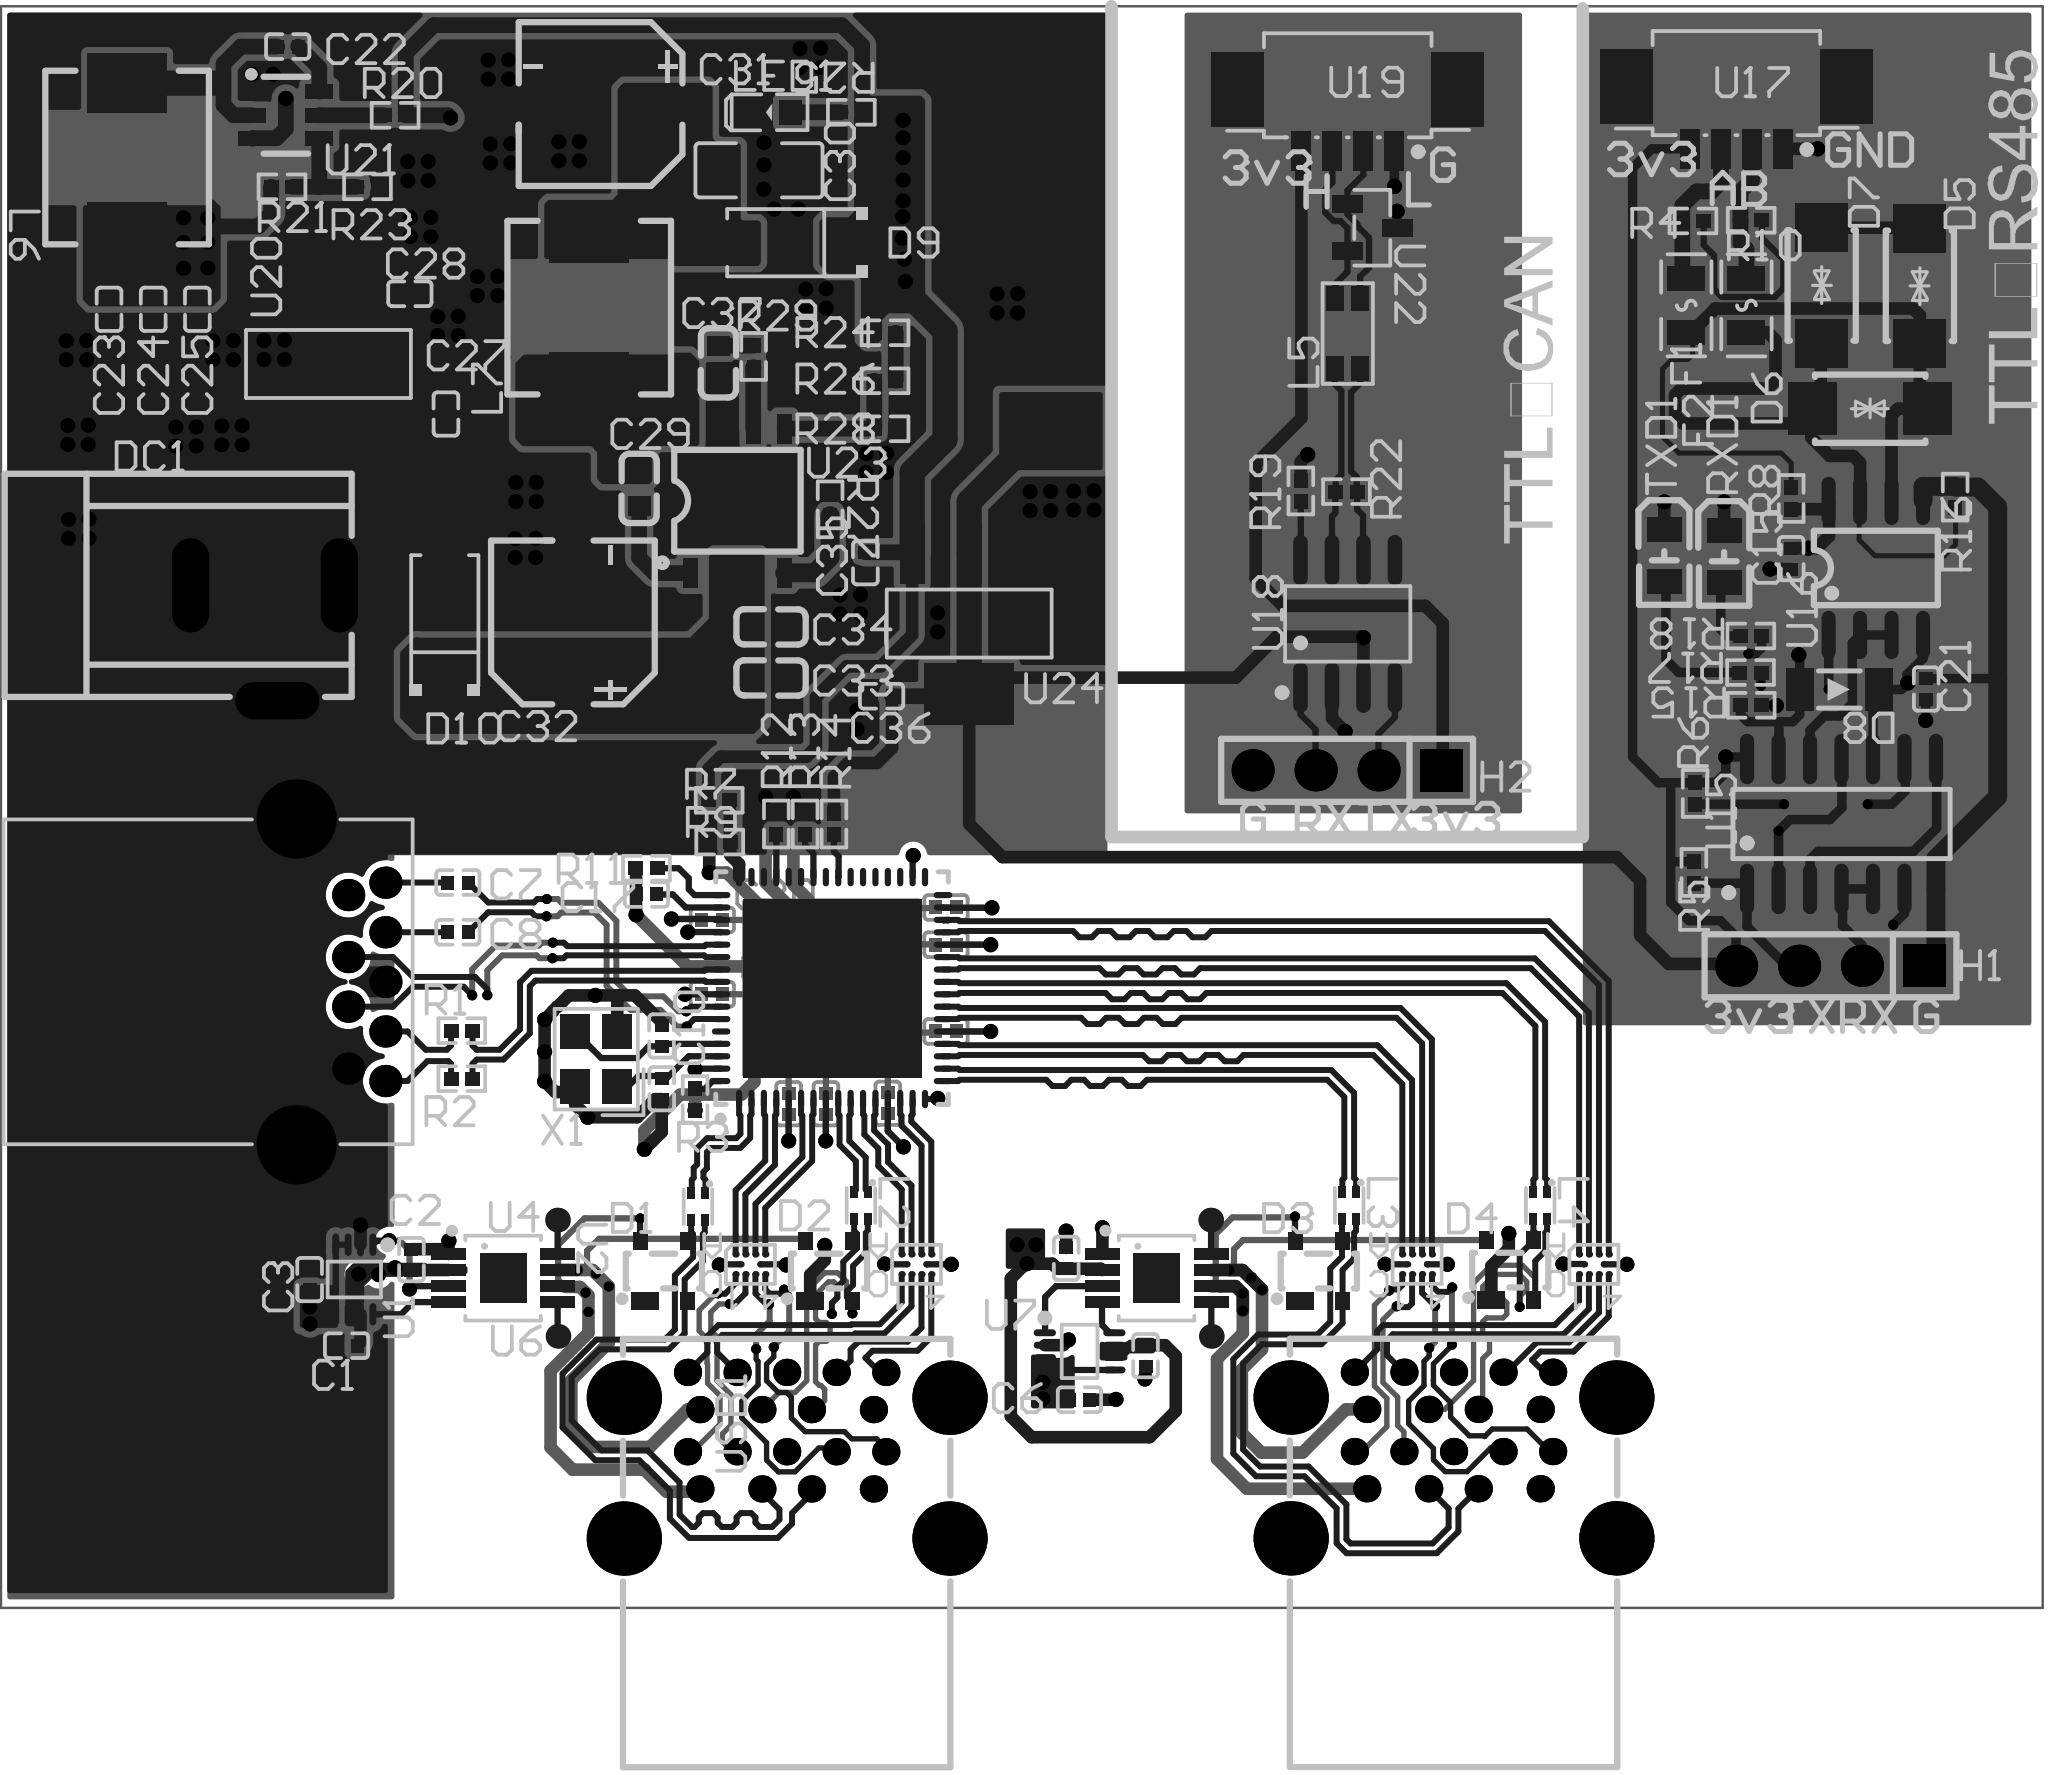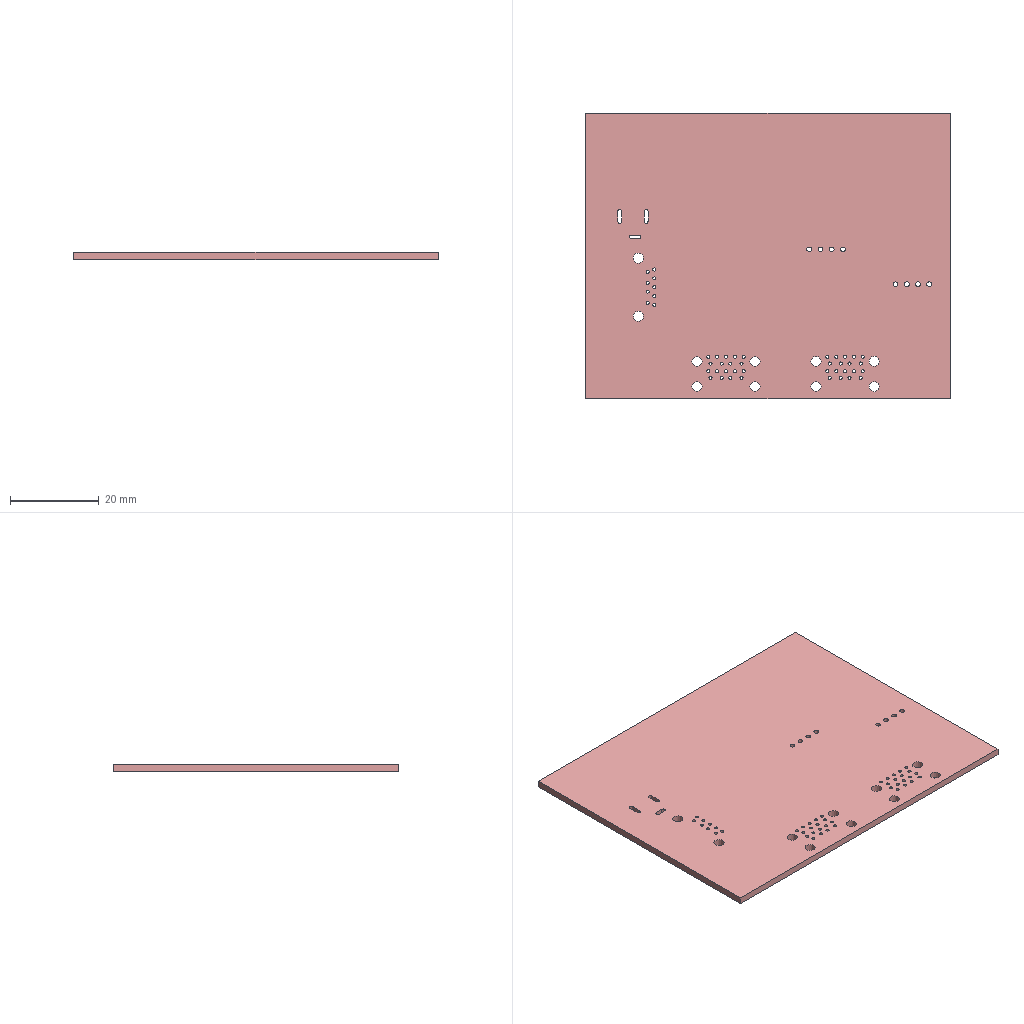Circuit board layout | Altium Designer | box 82.4 x 64.6 x 1.6 mm
Layer stack:
# Altium Designer layer stack of  (unit mm; dielectric type: 0 none, 1 core, 2 prepreg, 3 surface material)
index,name,kind,layer,copper_thickness_mm,dielectric_type,dielectric_thickness_mm,dielectric_material,dielectric_constant
0,Top Paste Mask Layer,other,,,,,,
1,Top Silkscreen Layer,other,,,,,,
2,Top Solder Mask Layer,dielectric,,,3,0,,0
3,Top Layer,copper,Top Layer,0.035,,,,
4,Dielectric1,dielectric,,,3,0.2104,7628 RC49% 8.6mil,0
5,GND,copper,GND,0.0152,,,,
6,Dielectric2,dielectric,,,3,1.065,1.1mm H/HOZ Copper,0
7,Signal-1,copper,Signal-1,0.0152,,,,
8,Dielectric3,dielectric,,,3,0.2104,7628 RC49% 8.6mil,0
9,Bottom Layer,copper,Bottom Layer,0.035,,,,
10,Bottom Solder Mask Layer,dielectric,,,3,0,,0
11,Bottom Silkscreen Layer,other,,,,,,
12,Bottom Paste Mask Layer,other,,,,,,
# drill layer pairs: low layer,high layer
drill_pair,Top Layer,Bottom Layer
Part placement:
Designator,Comment,Layer,Footprint,Center-X(mm),Center-Y(mm),Rotation
USB2,HC-USB3.0-L175-2X1-P,TopLayer,USB-A-TH_H181-AF2R06-12ALCR,134.993,88.908,0
U14,TUSB8041IRGCR,TopLayer,QFN-64_L9.0-W9.0-P0.50-BL-EP7.2,109.921,107.749,0
D4,CD143A-SR05,TopLayer,SOT-143_L2.9-W1.3-P1.92-LS2.3-BL,137.269,96.375,0
USB1,HC-USB3.0-L175-2X1-P,TopLayer,USB-A-TH_H181-AF2R06-12ALCR,108.09,88.9,0
L1,DLM11SN900HY2L,TopLayer,FILTER-SMD_4P-L1.3-W1.0-TL_DLP11SN201HL2L,104.511,98.936,270
U11,,TopLayer,PCMF2USB3S,133.524,96.609,90
C5,100nF,TopLayer,C0402,119.367,96.85,90
L3,DLM11SN900HY2L,TopLayer,FILTER-SMD_4P-L1.3-W1.0-TL_DLP11SN201HL2L,130.785,98.986,270
C31,220uF,TopLayer,CAP-SMD_BD6.3-L6.5-W6.5-LS7.2-FD,100.581,143.401,180
C32,100uF,TopLayer,CAP-SMD_BD6.3-L6.5-W6.5-LS7.0-FD,99.466,122.497,90
C30,47uF,TopLayer,C1206,106.972,140.729,180
C29,100nF,TopLayer,C0603,102.136,127.893,270
C34,100nF,TopLayer,C0603,107.452,122.319,180
C37,4.7nF,TopLayer,C0603,105.334,132.956,270
C33,4.7uF,TopLayer,C0603,107.452,120.259,180
D9,SS54,TopLayer,SMA_L4.4-W2.8-LS5.4-R-RD,108.336,137.81,180
D10,SS54,TopLayer,SMA_L4.4-W2.8-LS5.4-R-RD,94.297,122.563,90
D1,CD143A-SR05,TopLayer,SOT-143_L2.9-W1.3-P1.92-LS2.3-BL,103.124,96.337,0
D2,CD143A-SR05,TopLayer,SOT-143_L2.9-W1.3-P1.92-LS2.3-BL,109.789,96.337,0
D3,CD143A-SR05,TopLayer,SOT-143_L2.9-W1.3-P1.92-LS2.3-BL,129.548,96.337,0
D8,LL4148,TopLayer,LL-34_L3.5-W1.5-RD,150.557,119.791,180
D5,SMAJ6.5CA,TopLayer,SMA-L4.3-W2.6-LS5.3-BI,153.808,136.072,90
D7,SMAJ6.5CA,TopLayer,SMA-L4.3-W2.6-LS5.3-BI,149.846,136.085,270
D6,SMAJ6.5CA,TopLayer,SMA-L4.3-W2.6-LS5.3-BI,151.803,131.115,0
DC1,DC-005-A200,TopLayer,DC-IN-TH_DC-005-A200,87.041,121.666,0
H2,PZ254V-11-04P,TopLayer,HDR-TH_4P-P2.54-V-M,130.699,116.532,180
H1,PZ254V-11-04P,TopLayer,HDR-TH_4P-P2.54-V-M,150.203,108.648,180
L7,4.7uH,TopLayer,IND-SMD_L7.0-W6.6,100.124,135.192,90
L6,3.3uH,TopLayer,IND-SMD_L7.0-W6.6,81.481,141.244,90
L2,DLM11SN900HY2L,TopLayer,FILTER-SMD_4P-L1.3-W1.0-TL_DLP11SN201HL2L,111.087,98.986,270
L4,DLM11SN900HY2L,TopLayer,FILTER-SMD_4P-L1.3-W1.0-TL_DLP11SN201HL2L,138.491,98.986,270
L5,744232102,TopLayer,IND-SMD_4P-L3.2-W1.6,130.725,134.147,90
LED1,15-21VGC/TR8,TopLayer,LED0603_GREEN,107.391,143.071,180
RXD1,GL0805UR01,TopLayer,LED0805-R-RD_RED,145.909,125.163,270
TXD1,GL0805UR01,TopLayer,LED0805-R-RD_RED,143.496,125.201,270
U23,SCT2450STER,TopLayer,ESOP-8_L4.9-W3.9-P1.27-LS6.0-BL-EP,106.103,127.404,0
U21,TPS563201DDCR,TopLayer,SOT-23-6_L2.9-W1.6-P0.95-LS2.8-BR,87.884,142.951,180
U2,TPS2060CDGNR,TopLayer,HVSSOP-8_L3.0-W3.0-P0.65-LS4.9-BL-EP-1,96.65,96.053,270
U1,TXS0102DCUT,TopLayer,VSSOP-8_L2.3-W2.0-P0.50-LS3.1-BR,90.647,95.997,90
U8,TPS2060CDGNR,TopLayer,HVSSOP-8_L3.0-W3.0-P0.65-LS4.9-BL-EP-1,123.012,96.053,270
U7,TXS0102DCUT,TopLayer,VSSOP-8_L2.3-W2.0-P0.50-LS3.1-BR,119.908,93.098,180
U3,,TopLayer,PCMF2USB3S,113.329,96.609,90
U9,,TopLayer,PCMF2USB3S,140.658,96.609,90
U5,,TopLayer,PCMF2USB3S,106.629,96.609,90
U16,SP3485EN-L/TR,TopLayer,SOIC-8_L5.0-W4.0-P1.27-LS6.0-BL,152.03,124.693,0
U15,74HC04D,653,TopLayer,SOIC-14_L8.7-W3.9-P1.27-LS6.0-BL,150.646,114.368,0
U17,ZX-MX1.25-4PWT,TopLayer,CONN-SMD_4P-P1.25-MX1.25-4P-WT,146.404,142.846,180
U19,ZX-MX1.25-4PWT,TopLayer,CONN-SMD_4P-P1.25-MX1.25-4P-WT,130.725,142.757,180
U18,SN65HVD230DR,TopLayer,SOIC-8_L4.9-W3.9-P1.27-LS6.0-BL,130.725,122.437,0
U22,SM24CANA-02HTG,TopLayer,SOT-23-3_L2.9-W1.3-P1.90-LS2.4-BR,131.715,138.414,180
U13,HC-USB3.0-L168-WP,TopLayer,USB-TH_USB3.0-A,90.1,108.001,270
U20,AMS1117-1.8,TopLayer,SOT-223-4_L6.5-W3.5-P2.30-LS7.0-BR,89.604,132.918,270
U24,AMS1117-3.3,TopLayer,SOT-223-4_L6.5-W3.5-P2.30-LS7.0-BR,115.453,122.451,90
X1,24MHz,TopLayer,CRYSTAL-SMD_4P-L3.2-W2.5-BL,100.406,104.882,90
C22,100nF,TopLayer,C0402,87.96,145.72,0
C23,22uF,TopLayer,C0402,80.752,135.125,90
C24,22uF,TopLayer,C0402,82.534,135.125,90
C25,100nF,TopLayer,C0402,84.315,135.125,90
C10,12pF,TopLayer,C0402,103.04,105.819,270
C9,12pF,TopLayer,C0402,103.048,103.69,90
C17,100nF,TopLayer,C0402,102.433,111.524,180
C20,100nF,BottomLayer,C0402,105.09,110.498,180
C19,100nF,BottomLayer,C0402,109.672,103.086,270
C18,100nF,BottomLayer,C0402,114.517,109.499,0
C16,100nF,BottomLayer,C0402,114.517,111.001,0
C14,100nF,BottomLayer,C0402,114.517,105.999,0
C13,100nF,BottomLayer,C0402,112.169,103.104,270
C12,100nF,BottomLayer,C0402,105.09,107.5,180
C11,100nF,BottomLayer,C0402,108.168,103.086,270
C2,100nF,TopLayer,C0402,92.951,96.799,90
C1,100nF,TopLayer,C0402,90.335,93.327,0
C3,100nF,TopLayer,C0402,88.844,95.994,90
C4,100nF,TopLayer,C0402,122.568,92.926,90
C6,100nF,TopLayer,C0402,119.901,91.148,0
C15,Cap,TopLayer,C0402,148.615,125.07,270
C21,Cap,TopLayer,C0402,154.064,119.812,270
C8,100nF,TopLayer,C0402,94.825,110.002,0
C7,100nF,TopLayer,C0402,94.825,112.006,0
C28,22uF,TopLayer,C0402,92.888,135.75,180
C27,10uF,TopLayer,C0402,94.343,130.9,270
C36,22uF,TopLayer,C0402,111.92,119.52,0
C35,10uF,TopLayer,C0402,111.265,124.904,90
R26,1.5kΩ,TopLayer,R0402,112.057,132.241,180
R25,4.7kΩ,TopLayer,R0402,110.698,143.071,180
R28,10kΩ,TopLayer,R0402,112.057,130.304,0
R24,51kΩ,TopLayer,R0402,112.057,134.178,0
R29,20kΩ,TopLayer,R0402,106.756,133.223,90
R27,200kΩ,TopLayer,R0402,109.842,127.238,270
R20,10kΩ,TopLayer,R0402,92.293,142.949,0
R21,4.3kΩ,TopLayer,R0402,87.729,140.063,180
R23,10kΩ,TopLayer,R0402,91.178,140.063,0
R3,9.53K,TopLayer,R0402,104.394,103.251,270
R11,4.7K,TopLayer,R0402,102.433,112.583,180
R7,90.9K,TopLayer,R0402,105.367,115.323,180
R9,10K,TopLayer,R0402,105.389,113.637,180
R12,4.7K,TopLayer,R0402,107.673,114.366,90
R13,4.7K,TopLayer,R0402,108.834,114.366,90
R14,4.7K,TopLayer,R0402,109.997,114.366,90
R8,Res1,TopLayer,R0402,148.615,127.495,270
R16,Res1,TopLayer,R0402,155.231,127.549,270
R15,Res1,TopLayer,R0402,147.002,119.156,180
R17,Res1,TopLayer,R0402,146.976,120.476,180
R18,Res1,TopLayer,R0402,146.988,121.95,0
R5,Res1,TopLayer,R0402,144.69,112.412,90
R6,Res1,TopLayer,R0402,144.741,115.6,90
R10,Res1,TopLayer,R0402,147.001,138.714,0
R4,Res1,TopLayer,R0402,144.652,138.688,0
R19,10K,TopLayer,R0402,128.832,127.797,90
R22,120R 1%,TopLayer,R0402,130.674,127.771,180
R1,0R,TopLayer,R0402,94.982,106.032,0
R2,0R,TopLayer,R0402,94.982,104.096,0
U12,,TopLayer,tp点,125.222,93.703,180
U6,,TopLayer,tp点,98.864,93.703,0
U10,,TopLayer,tp点,125.197,98.394,180
U4,,TopLayer,tp点,98.844,98.394,0
F1,SMD0805-010-33,TopLayer,F0805,144.385,135.285,90
F2,SMD0805-010-33,TopLayer,F0805,146.811,135.285,90
Pad and via stacks:
# Altium Designer via and pad stacks of  (unit mm). Each distinct definition once, with the count of objects using it.
# via: kind,start_layer,end_layer,hole_mm,diameter_mm,mode(0 simple;1 top-mid-bottom;2 full stack),diameter_per_layer,count,example_net
# pad: kind,layer,hole_mm,hole_type(0 round;1 square;2 slot),plating,top_size,top_shape(1 round;2 rect;3 octagon;9 rounded rect),mid_size,bottom_size,mode,footprint,size_per_layer,count,example
pad,Multi-Layer,2.3,0,plated,3x3,1,3x3,3x3,0,USB-A-TH_H181-AF2R06-12ALCR,,8,USB2.20
pad,Multi-Layer,0.7,0,plated,1.1x1.1,1,1.1x1.1,1.1x1.1,0,USB-A-TH_H181-AF2R06-12ALCR,,36,USB2.18
pad,Multi-Layer,0.9,2,plated,1.5x3.8,1,1.5x3.8,1.5x3.8,0,DC-IN-TH_DC-005-A200,,2,DC1.1
pad,Multi-Layer,0.9,2,plated,1.5x3.4,1,1.5x3.4,1.5x3.4,0,DC-IN-TH_DC-005-A200,,1,DC1.3
pad,Multi-Layer,1.1,0,plated,1.7x1.7,2,1.7x1.7,1.7x1.7,0,HDR-TH_4P-P2.54-V-M,,2,H2.1
pad,Multi-Layer,1.1,0,plated,1.7x1.7,1,1.7x1.7,1.7x1.7,0,HDR-TH_4P-P2.54-V-M,,6,H2.2
pad,Multi-Layer,2.3,0,plated,3.2x3.2,1,3.2x3.2,3.2x3.2,0,USB-TH_USB3.0-A,,2,U13.10
pad,Multi-Layer,0.7,0,plated,1.3x1.3,1,1.3x1.3,1.3x1.3,0,USB-TH_USB3.0-A,,9,U13.9
pad,Top Layer,0,0,plated,0.25x0.75,1,0.25x0.75,0.25x0.75,0,QFN-64_L9.0-W9.0-P0.50-BL-EP7.2,,32,U14.1
pad,Top Layer,0,0,plated,7.2x7.2,2,7.2x7.2,7.2x7.2,0,QFN-64_L9.0-W9.0-P0.50-BL-EP7.2,,1,U14.65
pad,Top Layer,0,0,plated,0.7501x0.2499,1,0.7501x0.2499,0.7501x0.2499,0,QFN-64_L9.0-W9.0-P0.50-BL-EP7.2,,32,U14.31
pad,Top Layer,0,0,plated,1.1x0.7,2,1.1x0.7,1.1x0.7,0,SOT-143_L2.9-W1.3-P1.92-LS2.3-BL,,4,D4.1
pad,Top Layer,0,0,plated,0.6x0.7,2,0.6x0.7,0.6x0.7,0,SOT-143_L2.9-W1.3-P1.92-LS2.3-BL,,12,D4.2
pad,Top Layer,0,0,plated,0.465x0.308,2,0.465x0.308,0.465x0.308,0,FILTER-SMD_4P-L1.3-W1.0-TL_DLP11SN201HL2L,,16,L1.1
pad,Top Layer,0,0,unplated,0.254x0.254,1,0.254x0.254,0.254x0.254,0,PCMF2USB3S,,40,U11.C4
pad,Top Layer,0,0,plated,0.5x0.54,2,0.5x0.54,0.5x0.54,0,C0402,,42,C5.2
pad,Top Layer,0,0,plated,3.5x1.2,2,3.5x1.2,3.5x1.2,0,CAP-SMD_BD6.3-L6.5-W6.5-LS7.2-FD,,2,C31.1
pad,Top Layer,0,0,plated,3.5x1.2,2,3.5x1.2,3.5x1.2,0,CAP-SMD_BD6.3-L6.5-W6.5-LS7.0-FD,,2,C32.2
pad,Top Layer,0,0,plated,1.485x1.728,2,1.485x1.728,1.485x1.728,0,C1206,,2,C30.2
pad,Top Layer,0,0,plated,0.8x0.9,2,0.8x0.9,0.8x0.9,0,C0603,,8,C29.2
pad,Top Layer,0,0,plated,2.062x1.539,2,2.062x1.539,2.062x1.539,0,SMA_L4.4-W2.8-LS5.4-R-RD,,4,D9.1
pad,Top Layer,0,0,plated,1.1x1.7,2,1.1x1.7,1.1x1.7,0,LL-34_L3.5-W1.5-RD,,2,D8.2
pad,Top Layer,0,0,plated,1.96x2.1,2,1.96x2.1,1.96x2.1,0,SMA-L4.3-W2.6-LS5.3-BI,,6,D5.1
pad,Top Layer,0,0,plated,2.4x3.2,2,2.4x3.2,2.4x3.2,0,IND-SMD_L7.0-W6.6,,4,L7.1
pad,Top Layer,0,0,plated,1x0.7,2,1x0.7,1x0.7,0,IND-SMD_4P-L3.2-W1.6,,4,L5.4
pad,Top Layer,0,0,plated,1x0.8999,2,1x0.8999,1x0.8999,0,LED0603_GREEN,,2,LED1.2
pad,Top Layer,0,0,plated,1x1.399,2,1x1.399,1x1.399,0,LED0805-R-RD_RED,,4,RXD1.2
pad,Top Layer,0,0,plated,0.6x1.2,2,0.6x1.2,0.6x1.2,0,ESOP-8_L4.9-W3.9-P1.27-LS6.0-BL-EP,,8,U23.1
pad,Top Layer,0,0,plated,3.3x2.4,2,3.3x2.4,3.3x2.4,0,ESOP-8_L4.9-W3.9-P1.27-LS6.0-BL-EP,,1,U23.9
pad,Top Layer,0,0,plated,1.1x0.6,2,1.1x0.6,1.1x0.6,0,SOT-23-6_L2.9-W1.6-P0.95-LS2.8-BR,,6,U21.3
pad,Top Layer,0,0,plated,2x1.88,2,2x1.88,2x1.88,0,HVSSOP-8_L3.0-W3.0-P0.65-LS4.9-BL-EP-1,,2,U2.9
pad,Top Layer,0,0,plated,0.45x1.4,2,0.45x1.4,0.45x1.4,0,HVSSOP-8_L3.0-W3.0-P0.65-LS4.9-BL-EP-1,,16,U2.8
pad,Top Layer,0,0,plated,0.28x0.905,1,0.28x0.905,0.28x0.905,0,VSSOP-8_L2.3-W2.0-P0.50-LS3.1-BR,,16,U1.5
pad,Top Layer,0,0,plated,0.5684x1.95,1,0.5684x1.95,0.5684x1.95,0,SOIC-8_L5.0-W4.0-P1.27-LS6.0-BL,,8,U16.1
pad,Top Layer,0,0,plated,0.574x2.038,1,0.574x2.038,0.574x2.038,0,SOIC-14_L8.7-W3.9-P1.27-LS6.0-BL,,14,U15.8
pad,Top Layer,0,0,plated,2.1x3,2,2.1x3,2.1x3,0,CONN-SMD_4P-P1.25-MX1.25-4P-WT,,4,U17.6
pad,Top Layer,0,0,plated,0.8x1.6,2,0.8x1.6,0.8x1.6,0,CONN-SMD_4P-P1.25-MX1.25-4P-WT,,8,U17.4
pad,Top Layer,0,0,plated,0.588x2.045,1,0.588x2.045,0.588x2.045,0,SOIC-8_L4.9-W3.9-P1.27-LS6.0-BL,,8,U18.5
pad,Top Layer,0,0,plated,1.25x0.7,2,1.25x0.7,1.25x0.7,0,SOT-23-3_L2.9-W1.3-P1.90-LS2.4-BR,,3,U22.1
pad,Top Layer,0,0,plated,2.47x0.98,2,2.47x0.98,2.47x0.98,0,SOT-223-4_L6.5-W3.5-P2.30-LS7.0-BR,,6,U20.1
pad,Top Layer,0,0,plated,2.47x3.6,2,2.47x3.6,2.47x3.6,0,SOT-223-4_L6.5-W3.5-P2.30-LS7.0-BR,,2,U20.4
pad,Top Layer,0,0,plated,1.4x1.2,2,1.4x1.2,1.4x1.2,0,CRYSTAL-SMD_4P-L3.2-W2.5-BL,,4,X1.1
pad,Top Layer,0,0,plated,0.5657x0.54,2,0.5657x0.54,0.5657x0.54,0,R0402,,58,R26.2
pad,Top Layer,0,0,plated,1x1,1,1x1,1x1,0,tp\u00B5\u00E3,,4,U12.1
pad,Top Layer,0,0,plated,1x1.5,2,1x1.5,1x1.5,0,F0805,,4,F1.2
pad,Bottom Layer,0,0,plated,0.5x0.54,2,0.5x0.54,0.5x0.54,0,C0402,,16,C20.2
via,Top Layer,Bottom Layer,0.3048,0.4064,0,,47,$1N3880
via,Top Layer,Bottom Layer,0.3048,0.61,0,,276,GND
via,Top Layer,Bottom Layer,0.4064,0.6096,0,,1,3.3V
Copper pours:
name,layer,net,type(0 solid;1 hatched;2 none)
Signal-1-1.8V,Signal-1,1.8V,0
Signal-1-D5.0V,Signal-1,D5.0V,0
Signal-1-1.1V,Signal-1,1.1V,0
Signal-1-GND,Signal-1,GND,0
Signal-1-3.3V,Signal-1,3.3V,0
Top Layer-GND,Top Layer,GND,0
Top Layer-12V,Top Layer,12V,0
Top Layer-$1N10192,Top Layer,$1N10192,0
Top Layer-$1N10194,Top Layer,$1N10194,0
Top Layer-$1N10186,Top Layer,$1N10186,0
Top Layer-D5.0V,Top Layer,D5.0V,0
Top Layer-1.1V,Top Layer,1.1V,0
Top Layer-3.3V,Top Layer,3.3V,0
Top Layer-1.8V,Top Layer,1.8V,0
Top Layer-D5.0V 1,Top Layer,D5.0V,0
Top Layer-1.8V 1,Top Layer,1.8V,0
Top Layer-1.8V 2,Top Layer,1.8V,0
Top Layer-D5.0V 2,Top Layer,D5.0V,0
Top Layer-D5.0V 3,Top Layer,D5.0V,0
Bottom Layer-GND,Bottom Layer,GND,0
Bottom Layer-GND 1,Bottom Layer,GND,0
Bottom Layer-GND 2,Bottom Layer,GND,0
Bottom Layer-GND 3,Bottom Layer,GND,0
Bottom Layer-GND 4,Bottom Layer,GND,0
Design rules, without the lines most boards share:
# Altium Designer design rules of  (exported by Altium Designer, unit mm)
# columns: name | kind | enabled | priority | scope1 | scope2 | descriptor | typed fields (field=value)
Copper_copperRegion | 0 | disabled | 2 | All | All | Clearance Constraint (Gap=5.984mil) (Disabled)(All),(All) | gap=0.152
Copper_copperRegion_1 | 63 | disabled | 2 | All | All | Board Clearance Constraint (Gap=0mil) (Disabled)(All) |
Plane_innerPlane | 0 | disabled | 3 | All | All | Clearance Constraint (Gap=5.984mil) (Disabled)(All),(All) | gap=0.152
Plane_innerPlane_1 | 63 | disabled | 3 | All | All | Board Clearance Constraint (Gap=0mil) (Disabled)(All) |
copperThickness1oz_2 | 2 | enabled | 2 | All | All | Width Constraint (Min=3.9mil) (Max=100mil) (Preferred=20mil) (All) |
CAN | 51 | disabled | 1 | All | All | Differential Pairs Uncoupled Length using the Gap Constraints (Min=6mil) (Max=8mil) (Prefered=8mil)  and Width Constraints (Min=5mil) (Max=100mil) (Prefered=8mil) (Disabled)(All) |
usb2.0 | 51 | enabled | 2 | (InNet('USB30_T_DP1') OR InNet('$1N3807') OR InNet('$1N3806') OR InNet('$1N3821') OR InNet('$1N3814') OR InNet('$1N3813') OR InNet('$1N3822') OR InNet('$1N3831') OR InNet('$1N3827') OR InNet('USB30_T_DM1') OR InNet('USB30_T_DP2') OR InNet('USB30_T_DM2') OR InNet('USB30_T_DP3') OR InNet('USB30_T_DM3') OR InNet('USB30_T_DP4') OR InNet('USB30_T_DM4') OR InNet('USB30_USB_DM') OR InNet('USB30_USB_DP')) | All | Differential Pairs Uncoupled Length using the Gap Constraints (Min=5mil) (Max=6mil) (Prefered=6mil)  and Width Constraints (Min=8.4mil) (Max=9.5mil) (Prefered=9.5mil) ((InNet('USB30_T_DP1') OR InNet('$1N3807') OR InNet('$1N3806') OR InNet('$1N3821') OR InNet('$1N3814') OR InNet('$1N3813') OR InNet('$1N3822') OR InNet('$1N3831') OR InNet('$1N3827') OR InNet('USB30_T_DM1') OR InNet('USB30_T_DP2') OR InNet('USB30_T_DM2') OR InNet('USB30_T_DP3') OR InNet('USB30_T_DM3') OR InNet('USB30_T_DP4') OR InNet('USB30_T_DM4') OR InNet('USB30_USB_DM') OR InNet('USB30_USB_DP'))) |
usb3.0 | 51 | enabled | 3 | All | All | Differential Pairs Uncoupled Length using the Gap Constraints (Min=5mil) (Max=6mil) (Prefered=6mil)  and Width Constraints (Min=8.4mil) (Max=9.5mil) (Prefered=9.5mil) (All) |
RoutingVias | 11 | disabled | 1 | All | All | Routing Via (MinHoleWidth=5mil) (MaxHoleWidth=248.032mil) (PreferredHoleWidth=8mil) (MinWidth=10mil) (MaxWidth=393.701mil) (PreferedWidth=14mil) (Disabled)(All) | via_min_hole=0.127 via_max_hole=6.3 via_preferred_diameter=0.3556 via_preferred_hole=0.2032
viaSize | 11 | enabled | 2 | All | All | Routing Via (MinHoleWidth=11.811mil) (MaxHoleWidth=247.992mil) (PreferredHoleWidth=12.008mil) (MinWidth=15.748mil) (MaxWidth=100mil) (PreferedWidth=24.016mil) (All) | via_min_hole=0.3 via_max_hole=6.299 via_preferred_diameter=0.61 via_preferred_hole=0.305
innerPlane | 6 | enabled | 1 | All | All | Power Plane Connect Rule(Direct Connect )(Expansion=20mil) (Conductor Width=10mil) (Air Gap=10mil) (Entries=4) (All) | relief_conductor_width=0.254 relief_entries=4 relief_expansion=0.508
copperRegion | 20 | enabled | 1 | All | All | Polygon Connect Rule(Direct Connect )(Conductor Width=10mil) (Relief Angle=90 Angle) (Entries=4) (Air Gap Width=10mil) (All),(All) | connect_style(0=relief,1=direct,2=none)=1 relief_conductor_width=0.254 relief_entries=4
solderMaskExpansion | 13 | enabled | 2 | All | All | Solder Mask Expansion (Expansion =0.984mil) (All) | expansion=0.025